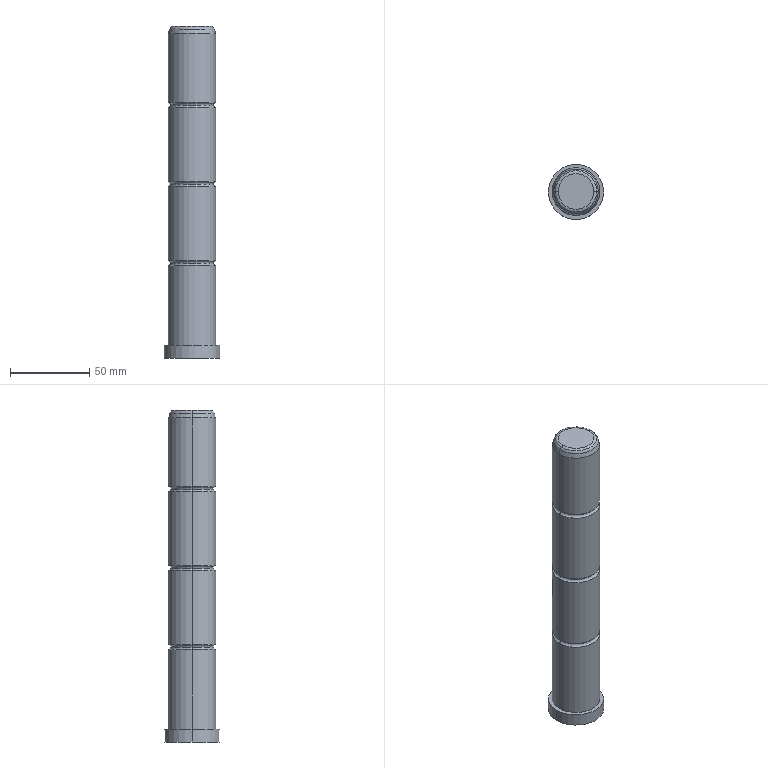Part | Creo | 1 solid | 37 faces | box 35 x 35 x 210 mm | volume 144944 mm3 | torus 16 | cylinder 12 | cone 6 | plane 3 | commonest cylinder face diameters 30 x8 12 x2 35 x2
STEP:
#1=CARTESIAN_POINT('',(-180.,-320.,-197.));
#2=VERTEX_POINT('',#1);
#3=CARTESIAN_POINT('',(-150.,-320.,-197.));
#4=VERTEX_POINT('',#3);
#5=CARTESIAN_POINT('',(-165.,-320.,-197.));
#6=DIRECTION('',(0.,0.,1.));
#7=DIRECTION('',(-1.,0.,0.));
#8=AXIS2_PLACEMENT_3D('',#5,#6,#7);
#9=CIRCLE('',#8,15.);
#10=EDGE_CURVE('',#2,#4,#9,.T.);
#11=ORIENTED_EDGE('',*,*,#10,.T.);
#12=CARTESIAN_POINT('',(-150.,-320.,-244.));
#13=VERTEX_POINT('',#12);
#14=CARTESIAN_POINT('',(-150.,-320.,-244.));
#15=DIRECTION('',(0.,0.,1.));
#16=VECTOR('',#15,47.);
#17=LINE('',#14,#16);
#18=EDGE_CURVE('',#13,#4,#17,.T.);
#19=ORIENTED_EDGE('',*,*,#18,.F.);
#20=CARTESIAN_POINT('',(-180.,-320.,-244.));
#21=VERTEX_POINT('',#20);
#22=CARTESIAN_POINT('',(-165.,-320.,-244.));
#23=DIRECTION('',(0.,0.,-1.));
#24=DIRECTION('',(1.,0.,0.));
#25=AXIS2_PLACEMENT_3D('',#22,#23,#24);
#26=CIRCLE('',#25,15.);
#27=EDGE_CURVE('',#13,#21,#26,.T.);
#28=ORIENTED_EDGE('',*,*,#27,.T.);
#29=CARTESIAN_POINT('',(-180.,-320.,-244.));
#30=DIRECTION('',(0.,0.,1.));
#31=VECTOR('',#30,47.);
#32=LINE('',#29,#31);
#33=EDGE_CURVE('',#21,#2,#32,.T.);
#34=ORIENTED_EDGE('',*,*,#33,.T.);
#35=EDGE_LOOP('',(#11,#19,#28,#34));
#36=FACE_OUTER_BOUND('',#35,.F.);
#37=CARTESIAN_POINT('',(-165.,-320.,-297.5));
#38=DIRECTION('',(0.,0.,1.));
#39=DIRECTION('',(-1.,0.,0.));
#40=AXIS2_PLACEMENT_3D('',#37,#38,#39);
#41=CYLINDRICAL_SURFACE('',#40,15.);
#42=ADVANCED_FACE('',(#36),#41,.T.);
#43=ORIENTED_EDGE('',*,*,#10,.F.);
#44=CARTESIAN_POINT('',(-178.5,-320.,-195.5));
#45=VERTEX_POINT('',#44);
#46=CARTESIAN_POINT('',(-180.,-320.,-195.5));
#47=DIRECTION('',(0.,1.,0.));
#48=DIRECTION('',(1.,0.,0.));
#49=AXIS2_PLACEMENT_3D('',#46,#47,#48);
#50=CIRCLE('',#49,1.5);
#51=EDGE_CURVE('',#45,#2,#50,.T.);
#52=ORIENTED_EDGE('',*,*,#51,.F.);
#53=CARTESIAN_POINT('',(-151.5,-320.,-195.5));
#54=VERTEX_POINT('',#53);
#55=CARTESIAN_POINT('',(-165.,-320.,-195.5));
#56=DIRECTION('',(0.,0.,1.));
#57=DIRECTION('',(-1.,0.,0.));
#58=AXIS2_PLACEMENT_3D('',#55,#56,#57);
#59=CIRCLE('',#58,13.5);
#60=EDGE_CURVE('',#45,#54,#59,.T.);
#61=ORIENTED_EDGE('',*,*,#60,.T.);
#62=CARTESIAN_POINT('',(-150.,-320.,-195.5));
#63=DIRECTION('',(0.,-1.,0.));
#64=DIRECTION('',(-1.,0.,0.));
#65=AXIS2_PLACEMENT_3D('',#62,#63,#64);
#66=CIRCLE('',#65,1.5);
#67=EDGE_CURVE('',#54,#4,#66,.T.);
#68=ORIENTED_EDGE('',*,*,#67,.T.);
#69=EDGE_LOOP('',(#43,#52,#61,#68));
#70=FACE_OUTER_BOUND('',#69,.F.);
#71=CARTESIAN_POINT('',(-165.,-320.,-195.5));
#72=DIRECTION('',(0.,0.,1.));
#73=DIRECTION('',(-1.,0.,0.));
#74=AXIS2_PLACEMENT_3D('',#71,#72,#73);
#75=TOROIDAL_SURFACE('',#74,15.,1.5);
#76=ADVANCED_FACE('',(#70),#75,.F.);
#77=CARTESIAN_POINT('',(-165.,-320.,-197.));
#78=DIRECTION('',(0.,0.,1.));
#79=DIRECTION('',(1.,0.,0.));
#80=AXIS2_PLACEMENT_3D('',#77,#78,#79);
#81=CIRCLE('',#80,15.);
#82=EDGE_CURVE('',#4,#2,#81,.T.);
#83=ORIENTED_EDGE('',*,*,#82,.F.);
#84=ORIENTED_EDGE('',*,*,#67,.F.);
#85=CARTESIAN_POINT('',(-165.,-320.,-195.5));
#86=DIRECTION('',(0.,0.,1.));
#87=DIRECTION('',(1.,0.,0.));
#88=AXIS2_PLACEMENT_3D('',#85,#86,#87);
#89=CIRCLE('',#88,13.5);
#90=EDGE_CURVE('',#54,#45,#89,.T.);
#91=ORIENTED_EDGE('',*,*,#90,.T.);
#92=ORIENTED_EDGE('',*,*,#51,.T.);
#93=EDGE_LOOP('',(#83,#84,#91,#92));
#94=FACE_OUTER_BOUND('',#93,.F.);
#95=CARTESIAN_POINT('',(-165.,-320.,-195.5));
#96=DIRECTION('',(0.,0.,1.));
#97=DIRECTION('',(-1.,0.,0.));
#98=AXIS2_PLACEMENT_3D('',#95,#96,#97);
#99=TOROIDAL_SURFACE('',#98,15.,1.5);
#100=ADVANCED_FACE('',(#94),#99,.F.);
#101=ORIENTED_EDGE('',*,*,#82,.T.);
#102=ORIENTED_EDGE('',*,*,#33,.F.);
#103=CARTESIAN_POINT('',(-165.,-320.,-244.));
#104=DIRECTION('',(0.,0.,-1.));
#105=DIRECTION('',(-1.,0.,0.));
#106=AXIS2_PLACEMENT_3D('',#103,#104,#105);
#107=CIRCLE('',#106,15.);
#108=EDGE_CURVE('',#21,#13,#107,.T.);
#109=ORIENTED_EDGE('',*,*,#108,.T.);
#110=ORIENTED_EDGE('',*,*,#18,.T.);
#111=EDGE_LOOP('',(#101,#102,#109,#110));
#112=FACE_OUTER_BOUND('',#111,.F.);
#113=CARTESIAN_POINT('',(-165.,-320.,-297.5));
#114=DIRECTION('',(0.,0.,1.));
#115=DIRECTION('',(-1.,0.,0.));
#116=AXIS2_PLACEMENT_3D('',#113,#114,#115);
#117=CYLINDRICAL_SURFACE('',#116,15.);
#118=ADVANCED_FACE('',(#112),#117,.T.);
#119=ORIENTED_EDGE('',*,*,#108,.F.);
#120=CARTESIAN_POINT('',(-178.5,-320.,-245.5));
#121=VERTEX_POINT('',#120);
#122=CARTESIAN_POINT('',(-180.,-320.,-245.5));
#123=DIRECTION('',(0.,1.,0.));
#124=DIRECTION('',(0.,0.,1.));
#125=AXIS2_PLACEMENT_3D('',#122,#123,#124);
#126=CIRCLE('',#125,1.5);
#127=EDGE_CURVE('',#21,#121,#126,.T.);
#128=ORIENTED_EDGE('',*,*,#127,.T.);
#129=CARTESIAN_POINT('',(-151.5,-320.,-245.5));
#130=VERTEX_POINT('',#129);
#131=CARTESIAN_POINT('',(-165.,-320.,-245.5));
#132=DIRECTION('',(0.,0.,1.));
#133=DIRECTION('',(1.,0.,0.));
#134=AXIS2_PLACEMENT_3D('',#131,#132,#133);
#135=CIRCLE('',#134,13.5);
#136=EDGE_CURVE('',#130,#121,#135,.T.);
#137=ORIENTED_EDGE('',*,*,#136,.F.);
#138=CARTESIAN_POINT('',(-150.,-320.,-245.5));
#139=DIRECTION('',(0.,-1.,0.));
#140=DIRECTION('',(0.,0.,1.));
#141=AXIS2_PLACEMENT_3D('',#138,#139,#140);
#142=CIRCLE('',#141,1.5);
#143=EDGE_CURVE('',#13,#130,#142,.T.);
#144=ORIENTED_EDGE('',*,*,#143,.F.);
#145=EDGE_LOOP('',(#119,#128,#137,#144));
#146=FACE_OUTER_BOUND('',#145,.F.);
#147=CARTESIAN_POINT('',(-165.,-320.,-245.5));
#148=DIRECTION('',(0.,0.,1.));
#149=DIRECTION('',(-1.,0.,0.));
#150=AXIS2_PLACEMENT_3D('',#147,#148,#149);
#151=TOROIDAL_SURFACE('',#150,15.,1.5);
#152=ADVANCED_FACE('',(#146),#151,.F.);
#153=ORIENTED_EDGE('',*,*,#27,.F.);
#154=ORIENTED_EDGE('',*,*,#143,.T.);
#155=CARTESIAN_POINT('',(-165.,-320.,-245.5));
#156=DIRECTION('',(0.,0.,1.));
#157=DIRECTION('',(-1.,0.,0.));
#158=AXIS2_PLACEMENT_3D('',#155,#156,#157);
#159=CIRCLE('',#158,13.5);
#160=EDGE_CURVE('',#121,#130,#159,.T.);
#161=ORIENTED_EDGE('',*,*,#160,.F.);
#162=ORIENTED_EDGE('',*,*,#127,.F.);
#163=EDGE_LOOP('',(#153,#154,#161,#162));
#164=FACE_OUTER_BOUND('',#163,.F.);
#165=CARTESIAN_POINT('',(-165.,-320.,-245.5));
#166=DIRECTION('',(0.,0.,1.));
#167=DIRECTION('',(-1.,0.,0.));
#168=AXIS2_PLACEMENT_3D('',#165,#166,#167);
#169=TOROIDAL_SURFACE('',#168,15.,1.5);
#170=ADVANCED_FACE('',(#164),#169,.F.);
#171=CARTESIAN_POINT('',(-180.,-320.,-247.));
#172=VERTEX_POINT('',#171);
#173=CARTESIAN_POINT('',(-150.,-320.,-247.));
#174=VERTEX_POINT('',#173);
#175=CARTESIAN_POINT('',(-165.,-320.,-247.));
#176=DIRECTION('',(0.,0.,1.));
#177=DIRECTION('',(-1.,0.,0.));
#178=AXIS2_PLACEMENT_3D('',#175,#176,#177);
#179=CIRCLE('',#178,15.);
#180=EDGE_CURVE('',#172,#174,#179,.T.);
#181=ORIENTED_EDGE('',*,*,#180,.F.);
#182=CARTESIAN_POINT('',(-180.,-320.,-245.5));
#183=DIRECTION('',(0.,1.,0.));
#184=DIRECTION('',(1.,0.,0.));
#185=AXIS2_PLACEMENT_3D('',#182,#183,#184);
#186=CIRCLE('',#185,1.5);
#187=EDGE_CURVE('',#121,#172,#186,.T.);
#188=ORIENTED_EDGE('',*,*,#187,.F.);
#189=ORIENTED_EDGE('',*,*,#160,.T.);
#190=CARTESIAN_POINT('',(-150.,-320.,-245.5));
#191=DIRECTION('',(0.,-1.,0.));
#192=DIRECTION('',(-1.,0.,0.));
#193=AXIS2_PLACEMENT_3D('',#190,#191,#192);
#194=CIRCLE('',#193,1.5);
#195=EDGE_CURVE('',#130,#174,#194,.T.);
#196=ORIENTED_EDGE('',*,*,#195,.T.);
#197=EDGE_LOOP('',(#181,#188,#189,#196));
#198=FACE_OUTER_BOUND('',#197,.F.);
#199=CARTESIAN_POINT('',(-165.,-320.,-245.5));
#200=DIRECTION('',(0.,0.,1.));
#201=DIRECTION('',(-1.,0.,0.));
#202=AXIS2_PLACEMENT_3D('',#199,#200,#201);
#203=TOROIDAL_SURFACE('',#202,15.,1.5);
#204=ADVANCED_FACE('',(#198),#203,.F.);
#205=CARTESIAN_POINT('',(-150.,-320.,-297.5));
#206=VERTEX_POINT('',#205);
#207=CARTESIAN_POINT('',(-180.,-320.,-297.5));
#208=VERTEX_POINT('',#207);
#209=CARTESIAN_POINT('',(-165.,-320.,-297.5));
#210=DIRECTION('',(0.,0.,-1.));
#211=DIRECTION('',(1.,0.,0.));
#212=AXIS2_PLACEMENT_3D('',#209,#210,#211);
#213=CIRCLE('',#212,15.);
#214=EDGE_CURVE('',#206,#208,#213,.T.);
#215=ORIENTED_EDGE('',*,*,#214,.T.);
#216=CARTESIAN_POINT('',(-180.,-320.,-297.5));
#217=DIRECTION('',(0.,0.,1.));
#218=VECTOR('',#217,50.5);
#219=LINE('',#216,#218);
#220=EDGE_CURVE('',#208,#172,#219,.T.);
#221=ORIENTED_EDGE('',*,*,#220,.T.);
#222=ORIENTED_EDGE('',*,*,#180,.T.);
#223=CARTESIAN_POINT('',(-150.,-320.,-297.5));
#224=DIRECTION('',(0.,0.,1.));
#225=VECTOR('',#224,50.5);
#226=LINE('',#223,#225);
#227=EDGE_CURVE('',#206,#174,#226,.T.);
#228=ORIENTED_EDGE('',*,*,#227,.F.);
#229=EDGE_LOOP('',(#215,#221,#222,#228));
#230=FACE_OUTER_BOUND('',#229,.F.);
#231=CARTESIAN_POINT('',(-165.,-320.,-297.5));
#232=DIRECTION('',(0.,0.,1.));
#233=DIRECTION('',(-1.,0.,0.));
#234=AXIS2_PLACEMENT_3D('',#231,#232,#233);
#235=CYLINDRICAL_SURFACE('',#234,15.);
#236=ADVANCED_FACE('',(#230),#235,.T.);
#237=CARTESIAN_POINT('',(-147.5,-320.,-297.5));
#238=VERTEX_POINT('',#237);
#239=CARTESIAN_POINT('',(-182.5,-320.,-297.5));
#240=VERTEX_POINT('',#239);
#241=CARTESIAN_POINT('',(-165.,-320.,-297.5));
#242=DIRECTION('',(0.,0.,1.));
#243=DIRECTION('',(1.,0.,0.));
#244=AXIS2_PLACEMENT_3D('',#241,#242,#243);
#245=CIRCLE('',#244,17.5);
#246=EDGE_CURVE('',#238,#240,#245,.T.);
#247=ORIENTED_EDGE('',*,*,#246,.F.);
#248=CARTESIAN_POINT('',(-165.,-320.,-297.5));
#249=DIRECTION('',(0.,0.,1.));
#250=DIRECTION('',(-1.,0.,0.));
#251=AXIS2_PLACEMENT_3D('',#248,#249,#250);
#252=CIRCLE('',#251,17.5);
#253=EDGE_CURVE('',#240,#238,#252,.T.);
#254=ORIENTED_EDGE('',*,*,#253,.F.);
#255=EDGE_LOOP('',(#247,#254));
#256=FACE_OUTER_BOUND('',#255,.F.);
#257=CARTESIAN_POINT('',(-165.,-320.,-297.5));
#258=DIRECTION('',(0.,0.,-1.));
#259=DIRECTION('',(-1.,0.,0.));
#260=AXIS2_PLACEMENT_3D('',#257,#258,#259);
#261=CIRCLE('',#260,15.);
#262=EDGE_CURVE('',#208,#206,#261,.T.);
#263=ORIENTED_EDGE('',*,*,#262,.F.);
#264=ORIENTED_EDGE('',*,*,#214,.F.);
#265=EDGE_LOOP('',(#263,#264));
#266=FACE_BOUND('',#265,.F.);
#267=CARTESIAN_POINT('',(-165.,-320.,-297.5));
#268=DIRECTION('',(0.,0.,-1.));
#269=DIRECTION('',(1.,0.,0.));
#270=AXIS2_PLACEMENT_3D('',#267,#268,#269);
#271=PLANE('',#270);
#272=ADVANCED_FACE('',(#256,#266),#271,.F.);
#273=ORIENTED_EDGE('',*,*,#262,.T.);
#274=ORIENTED_EDGE('',*,*,#227,.T.);
#275=CARTESIAN_POINT('',(-165.,-320.,-247.));
#276=DIRECTION('',(0.,0.,1.));
#277=DIRECTION('',(1.,0.,0.));
#278=AXIS2_PLACEMENT_3D('',#275,#276,#277);
#279=CIRCLE('',#278,15.);
#280=EDGE_CURVE('',#174,#172,#279,.T.);
#281=ORIENTED_EDGE('',*,*,#280,.T.);
#282=ORIENTED_EDGE('',*,*,#220,.F.);
#283=EDGE_LOOP('',(#273,#274,#281,#282));
#284=FACE_OUTER_BOUND('',#283,.F.);
#285=CARTESIAN_POINT('',(-165.,-320.,-297.5));
#286=DIRECTION('',(0.,0.,1.));
#287=DIRECTION('',(-1.,0.,0.));
#288=AXIS2_PLACEMENT_3D('',#285,#286,#287);
#289=CYLINDRICAL_SURFACE('',#288,15.);
#290=ADVANCED_FACE('',(#284),#289,.T.);
#291=ORIENTED_EDGE('',*,*,#280,.F.);
#292=ORIENTED_EDGE('',*,*,#195,.F.);
#293=ORIENTED_EDGE('',*,*,#136,.T.);
#294=ORIENTED_EDGE('',*,*,#187,.T.);
#295=EDGE_LOOP('',(#291,#292,#293,#294));
#296=FACE_OUTER_BOUND('',#295,.F.);
#297=CARTESIAN_POINT('',(-165.,-320.,-245.5));
#298=DIRECTION('',(0.,0.,1.));
#299=DIRECTION('',(-1.,0.,0.));
#300=AXIS2_PLACEMENT_3D('',#297,#298,#299);
#301=TOROIDAL_SURFACE('',#300,15.,1.5);
#302=ADVANCED_FACE('',(#296),#301,.F.);
#303=ORIENTED_EDGE('',*,*,#246,.T.);
#304=CARTESIAN_POINT('',(-182.5,-320.,-305.5));
#305=VERTEX_POINT('',#304);
#306=CARTESIAN_POINT('',(-182.5,-320.,-297.5));
#307=DIRECTION('',(0.,0.,-1.));
#308=VECTOR('',#307,8.);
#309=LINE('',#306,#308);
#310=EDGE_CURVE('',#240,#305,#309,.T.);
#311=ORIENTED_EDGE('',*,*,#310,.T.);
#312=CARTESIAN_POINT('',(-147.5,-320.,-305.5));
#313=VERTEX_POINT('',#312);
#314=CARTESIAN_POINT('',(-165.,-320.,-305.5));
#315=DIRECTION('',(0.,0.,-1.));
#316=DIRECTION('',(-1.,0.,0.));
#317=AXIS2_PLACEMENT_3D('',#314,#315,#316);
#318=CIRCLE('',#317,17.5);
#319=EDGE_CURVE('',#305,#313,#318,.T.);
#320=ORIENTED_EDGE('',*,*,#319,.T.);
#321=CARTESIAN_POINT('',(-147.5,-320.,-297.5));
#322=DIRECTION('',(0.,0.,-1.));
#323=VECTOR('',#322,8.);
#324=LINE('',#321,#323);
#325=EDGE_CURVE('',#238,#313,#324,.T.);
#326=ORIENTED_EDGE('',*,*,#325,.F.);
#327=EDGE_LOOP('',(#303,#311,#320,#326));
#328=FACE_OUTER_BOUND('',#327,.F.);
#329=CARTESIAN_POINT('',(-165.,-320.,-297.5));
#330=DIRECTION('',(0.,0.,-1.));
#331=DIRECTION('',(1.,0.,0.));
#332=AXIS2_PLACEMENT_3D('',#329,#330,#331);
#333=CYLINDRICAL_SURFACE('',#332,17.5);
#334=ADVANCED_FACE('',(#328),#333,.T.);
#335=ORIENTED_EDGE('',*,*,#253,.T.);
#336=ORIENTED_EDGE('',*,*,#325,.T.);
#337=CARTESIAN_POINT('',(-165.,-320.,-305.5));
#338=DIRECTION('',(0.,0.,-1.));
#339=DIRECTION('',(1.,0.,0.));
#340=AXIS2_PLACEMENT_3D('',#337,#338,#339);
#341=CIRCLE('',#340,17.5);
#342=EDGE_CURVE('',#313,#305,#341,.T.);
#343=ORIENTED_EDGE('',*,*,#342,.T.);
#344=ORIENTED_EDGE('',*,*,#310,.F.);
#345=EDGE_LOOP('',(#335,#336,#343,#344));
#346=FACE_OUTER_BOUND('',#345,.F.);
#347=CARTESIAN_POINT('',(-165.,-320.,-297.5));
#348=DIRECTION('',(0.,0.,-1.));
#349=DIRECTION('',(1.,0.,0.));
#350=AXIS2_PLACEMENT_3D('',#347,#348,#349);
#351=CYLINDRICAL_SURFACE('',#350,17.5);
#352=ADVANCED_FACE('',(#346),#351,.T.);
#353=ORIENTED_EDGE('',*,*,#342,.F.);
#354=ORIENTED_EDGE('',*,*,#319,.F.);
#355=EDGE_LOOP('',(#353,#354));
#356=FACE_OUTER_BOUND('',#355,.F.);
#357=CARTESIAN_POINT('',(-156.5,-320.,-305.5));
#358=VERTEX_POINT('',#357);
#359=CARTESIAN_POINT('',(-173.5,-320.,-305.5));
#360=VERTEX_POINT('',#359);
#361=CARTESIAN_POINT('',(-165.,-320.,-305.5));
#362=DIRECTION('',(0.,0.,1.));
#363=DIRECTION('',(1.,0.,0.));
#364=AXIS2_PLACEMENT_3D('',#361,#362,#363);
#365=CIRCLE('',#364,8.5);
#366=EDGE_CURVE('',#358,#360,#365,.T.);
#367=ORIENTED_EDGE('',*,*,#366,.F.);
#368=CARTESIAN_POINT('',(-165.,-320.,-305.5));
#369=DIRECTION('',(0.,0.,1.));
#370=DIRECTION('',(-1.,0.,0.));
#371=AXIS2_PLACEMENT_3D('',#368,#369,#370);
#372=CIRCLE('',#371,8.5);
#373=EDGE_CURVE('',#360,#358,#372,.T.);
#374=ORIENTED_EDGE('',*,*,#373,.F.);
#375=EDGE_LOOP('',(#367,#374));
#376=FACE_BOUND('',#375,.F.);
#377=CARTESIAN_POINT('',(-165.,-320.,-305.5));
#378=DIRECTION('',(0.,0.,-1.));
#379=DIRECTION('',(1.,0.,0.));
#380=AXIS2_PLACEMENT_3D('',#377,#378,#379);
#381=PLANE('',#380);
#382=ADVANCED_FACE('',(#356,#376),#381,.T.);
#383=CARTESIAN_POINT('',(-159.,-320.,-303.));
#384=VERTEX_POINT('',#383);
#385=CARTESIAN_POINT('',(-171.,-320.,-303.));
#386=VERTEX_POINT('',#385);
#387=CARTESIAN_POINT('',(-165.,-320.,-303.));
#388=DIRECTION('',(0.,0.,1.));
#389=DIRECTION('',(1.,0.,0.));
#390=AXIS2_PLACEMENT_3D('',#387,#388,#389);
#391=CIRCLE('',#390,6.);
#392=EDGE_CURVE('',#384,#386,#391,.T.);
#393=ORIENTED_EDGE('',*,*,#392,.F.);
#394=CARTESIAN_POINT('',(-159.,-320.,-303.));
#395=DIRECTION('',(0.7071,0.,-0.7071));
#396=VECTOR('',#395,3.536);
#397=LINE('',#394,#396);
#398=EDGE_CURVE('',#384,#358,#397,.T.);
#399=ORIENTED_EDGE('',*,*,#398,.T.);
#400=ORIENTED_EDGE('',*,*,#366,.T.);
#401=CARTESIAN_POINT('',(-171.,-320.,-303.));
#402=DIRECTION('',(-0.7071,0.,-0.7071));
#403=VECTOR('',#402,3.536);
#404=LINE('',#401,#403);
#405=EDGE_CURVE('',#386,#360,#404,.T.);
#406=ORIENTED_EDGE('',*,*,#405,.F.);
#407=EDGE_LOOP('',(#393,#399,#400,#406));
#408=FACE_OUTER_BOUND('',#407,.F.);
#409=CARTESIAN_POINT('',(-165.,-320.,-304.25));
#410=DIRECTION('',(0.,0.,-1.));
#411=DIRECTION('',(1.,0.,0.));
#412=AXIS2_PLACEMENT_3D('',#409,#410,#411);
#413=CONICAL_SURFACE('',#412,7.25,45.);
#414=ADVANCED_FACE('',(#408),#413,.F.);
#415=ORIENTED_EDGE('',*,*,#392,.T.);
#416=CARTESIAN_POINT('',(-171.,-320.,-271.087));
#417=VERTEX_POINT('',#416);
#418=CARTESIAN_POINT('',(-171.,-320.,-303.));
#419=DIRECTION('',(0.,0.,1.));
#420=VECTOR('',#419,31.913);
#421=LINE('',#418,#420);
#422=EDGE_CURVE('',#386,#417,#421,.T.);
#423=ORIENTED_EDGE('',*,*,#422,.T.);
#424=CARTESIAN_POINT('',(-159.,-320.,-271.087));
#425=VERTEX_POINT('',#424);
#426=CARTESIAN_POINT('',(-165.,-320.,-271.087));
#427=DIRECTION('',(0.,0.,-1.));
#428=DIRECTION('',(-1.,0.,0.));
#429=AXIS2_PLACEMENT_3D('',#426,#427,#428);
#430=CIRCLE('',#429,6.);
#431=EDGE_CURVE('',#417,#425,#430,.T.);
#432=ORIENTED_EDGE('',*,*,#431,.T.);
#433=CARTESIAN_POINT('',(-159.,-320.,-303.));
#434=DIRECTION('',(0.,0.,1.));
#435=VECTOR('',#434,31.913);
#436=LINE('',#433,#435);
#437=EDGE_CURVE('',#384,#425,#436,.T.);
#438=ORIENTED_EDGE('',*,*,#437,.F.);
#439=EDGE_LOOP('',(#415,#423,#432,#438));
#440=FACE_OUTER_BOUND('',#439,.F.);
#441=CARTESIAN_POINT('',(-165.,-320.,-305.5));
#442=DIRECTION('',(0.,0.,1.));
#443=DIRECTION('',(-1.,0.,0.));
#444=AXIS2_PLACEMENT_3D('',#441,#442,#443);
#445=CYLINDRICAL_SURFACE('',#444,6.);
#446=ADVANCED_FACE('',(#440),#445,.F.);
#447=CARTESIAN_POINT('',(-165.,-320.,-303.));
#448=DIRECTION('',(0.,0.,1.));
#449=DIRECTION('',(-1.,0.,0.));
#450=AXIS2_PLACEMENT_3D('',#447,#448,#449);
#451=CIRCLE('',#450,6.);
#452=EDGE_CURVE('',#386,#384,#451,.T.);
#453=ORIENTED_EDGE('',*,*,#452,.T.);
#454=ORIENTED_EDGE('',*,*,#437,.T.);
#455=CARTESIAN_POINT('',(-165.,-320.,-271.087));
#456=DIRECTION('',(0.,0.,-1.));
#457=DIRECTION('',(1.,0.,0.));
#458=AXIS2_PLACEMENT_3D('',#455,#456,#457);
#459=CIRCLE('',#458,6.);
#460=EDGE_CURVE('',#425,#417,#459,.T.);
#461=ORIENTED_EDGE('',*,*,#460,.T.);
#462=ORIENTED_EDGE('',*,*,#422,.F.);
#463=EDGE_LOOP('',(#453,#454,#461,#462));
#464=FACE_OUTER_BOUND('',#463,.F.);
#465=CARTESIAN_POINT('',(-165.,-320.,-305.5));
#466=DIRECTION('',(0.,0.,1.));
#467=DIRECTION('',(-1.,0.,0.));
#468=AXIS2_PLACEMENT_3D('',#465,#466,#467);
#469=CYLINDRICAL_SURFACE('',#468,6.);
#470=ADVANCED_FACE('',(#464),#469,.F.);
#471=ORIENTED_EDGE('',*,*,#452,.F.);
#472=ORIENTED_EDGE('',*,*,#405,.T.);
#473=ORIENTED_EDGE('',*,*,#373,.T.);
#474=ORIENTED_EDGE('',*,*,#398,.F.);
#475=EDGE_LOOP('',(#471,#472,#473,#474));
#476=FACE_OUTER_BOUND('',#475,.F.);
#477=CARTESIAN_POINT('',(-165.,-320.,-304.25));
#478=DIRECTION('',(0.,0.,-1.));
#479=DIRECTION('',(1.,0.,0.));
#480=AXIS2_PLACEMENT_3D('',#477,#478,#479);
#481=CONICAL_SURFACE('',#480,7.25,45.);
#482=ADVANCED_FACE('',(#476),#481,.F.);
#483=ORIENTED_EDGE('',*,*,#460,.F.);
#484=CARTESIAN_POINT('',(-165.,-320.,-267.482));
#485=VERTEX_POINT('',#484);
#486=CARTESIAN_POINT('',(-165.,-320.,-267.482));
#487=DIRECTION('',(0.8572,0.,-0.515));
#488=VECTOR('',#487,7.);
#489=LINE('',#486,#488);
#490=EDGE_CURVE('',#485,#425,#489,.T.);
#491=ORIENTED_EDGE('',*,*,#490,.F.);
#492=CARTESIAN_POINT('',(-165.,-320.,-267.482));
#493=DIRECTION('',(-0.8572,0.,-0.515));
#494=VECTOR('',#493,7.);
#495=LINE('',#492,#494);
#496=EDGE_CURVE('',#485,#417,#495,.T.);
#497=ORIENTED_EDGE('',*,*,#496,.T.);
#498=EDGE_LOOP('',(#483,#491,#497));
#499=FACE_OUTER_BOUND('',#498,.F.);
#500=CARTESIAN_POINT('',(-165.,-320.,-269.351));
#501=DIRECTION('',(0.,0.,-1.));
#502=DIRECTION('',(1.,0.,0.));
#503=AXIS2_PLACEMENT_3D('',#500,#501,#502);
#504=CONICAL_SURFACE('',#503,3.111,59.);
#505=ADVANCED_FACE('',(#499),#504,.F.);
#506=ORIENTED_EDGE('',*,*,#431,.F.);
#507=ORIENTED_EDGE('',*,*,#496,.F.);
#508=ORIENTED_EDGE('',*,*,#490,.T.);
#509=EDGE_LOOP('',(#506,#507,#508));
#510=FACE_OUTER_BOUND('',#509,.F.);
#511=CARTESIAN_POINT('',(-165.,-320.,-269.351));
#512=DIRECTION('',(0.,0.,-1.));
#513=DIRECTION('',(1.,0.,0.));
#514=AXIS2_PLACEMENT_3D('',#511,#512,#513);
#515=CONICAL_SURFACE('',#514,3.111,59.);
#516=ADVANCED_FACE('',(#510),#515,.F.);
#517=CARTESIAN_POINT('',(-180.,-320.,-194.));
#518=VERTEX_POINT('',#517);
#519=CARTESIAN_POINT('',(-150.,-320.,-194.));
#520=VERTEX_POINT('',#519);
#521=CARTESIAN_POINT('',(-165.,-320.,-194.));
#522=DIRECTION('',(0.,0.,-1.));
#523=DIRECTION('',(-1.,0.,0.));
#524=AXIS2_PLACEMENT_3D('',#521,#522,#523);
#525=CIRCLE('',#524,15.);
#526=EDGE_CURVE('',#518,#520,#525,.T.);
#527=ORIENTED_EDGE('',*,*,#526,.F.);
#528=CARTESIAN_POINT('',(-180.,-320.,-195.5));
#529=DIRECTION('',(0.,1.,0.));
#530=DIRECTION('',(0.,0.,1.));
#531=AXIS2_PLACEMENT_3D('',#528,#529,#530);
#532=CIRCLE('',#531,1.5);
#533=EDGE_CURVE('',#518,#45,#532,.T.);
#534=ORIENTED_EDGE('',*,*,#533,.T.);
#535=ORIENTED_EDGE('',*,*,#90,.F.);
#536=CARTESIAN_POINT('',(-150.,-320.,-195.5));
#537=DIRECTION('',(0.,-1.,0.));
#538=DIRECTION('',(0.,0.,1.));
#539=AXIS2_PLACEMENT_3D('',#536,#537,#538);
#540=CIRCLE('',#539,1.5);
#541=EDGE_CURVE('',#520,#54,#540,.T.);
#542=ORIENTED_EDGE('',*,*,#541,.F.);
#543=EDGE_LOOP('',(#527,#534,#535,#542));
#544=FACE_OUTER_BOUND('',#543,.F.);
#545=CARTESIAN_POINT('',(-165.,-320.,-195.5));
#546=DIRECTION('',(0.,0.,1.));
#547=DIRECTION('',(-1.,0.,0.));
#548=AXIS2_PLACEMENT_3D('',#545,#546,#547);
#549=TOROIDAL_SURFACE('',#548,15.,1.5);
#550=ADVANCED_FACE('',(#544),#549,.F.);
#551=CARTESIAN_POINT('',(-150.,-320.,-147.));
#552=VERTEX_POINT('',#551);
#553=CARTESIAN_POINT('',(-180.,-320.,-147.));
#554=VERTEX_POINT('',#553);
#555=CARTESIAN_POINT('',(-165.,-320.,-147.));
#556=DIRECTION('',(0.,0.,1.));
#557=DIRECTION('',(1.,0.,0.));
#558=AXIS2_PLACEMENT_3D('',#555,#556,#557);
#559=CIRCLE('',#558,15.);
#560=EDGE_CURVE('',#552,#554,#559,.T.);
#561=ORIENTED_EDGE('',*,*,#560,.T.);
#562=CARTESIAN_POINT('',(-180.,-320.,-194.));
#563=DIRECTION('',(0.,0.,1.));
#564=VECTOR('',#563,47.);
#565=LINE('',#562,#564);
#566=EDGE_CURVE('',#518,#554,#565,.T.);
#567=ORIENTED_EDGE('',*,*,#566,.F.);
#568=ORIENTED_EDGE('',*,*,#526,.T.);
#569=CARTESIAN_POINT('',(-150.,-320.,-194.));
#570=DIRECTION('',(0.,0.,1.));
#571=VECTOR('',#570,47.);
#572=LINE('',#569,#571);
#573=EDGE_CURVE('',#520,#552,#572,.T.);
#574=ORIENTED_EDGE('',*,*,#573,.T.);
#575=EDGE_LOOP('',(#561,#567,#568,#574));
#576=FACE_OUTER_BOUND('',#575,.F.);
#577=CARTESIAN_POINT('',(-165.,-320.,-297.5));
#578=DIRECTION('',(0.,0.,1.));
#579=DIRECTION('',(-1.,0.,0.));
#580=AXIS2_PLACEMENT_3D('',#577,#578,#579);
#581=CYLINDRICAL_SURFACE('',#580,15.);
#582=ADVANCED_FACE('',(#576),#581,.T.);
#583=ORIENTED_EDGE('',*,*,#560,.F.);
#584=CARTESIAN_POINT('',(-151.5,-320.,-145.5));
#585=VERTEX_POINT('',#584);
#586=CARTESIAN_POINT('',(-150.,-320.,-145.5));
#587=DIRECTION('',(0.,-1.,0.));
#588=DIRECTION('',(-1.,0.,0.));
#589=AXIS2_PLACEMENT_3D('',#586,#587,#588);
#590=CIRCLE('',#589,1.5);
#591=EDGE_CURVE('',#585,#552,#590,.T.);
#592=ORIENTED_EDGE('',*,*,#591,.F.);
#593=CARTESIAN_POINT('',(-178.5,-320.,-145.5));
#594=VERTEX_POINT('',#593);
#595=CARTESIAN_POINT('',(-165.,-320.,-145.5));
#596=DIRECTION('',(0.,0.,1.));
#597=DIRECTION('',(1.,0.,0.));
#598=AXIS2_PLACEMENT_3D('',#595,#596,#597);
#599=CIRCLE('',#598,13.5);
#600=EDGE_CURVE('',#585,#594,#599,.T.);
#601=ORIENTED_EDGE('',*,*,#600,.T.);
#602=CARTESIAN_POINT('',(-180.,-320.,-145.5));
#603=DIRECTION('',(0.,1.,0.));
#604=DIRECTION('',(1.,0.,0.));
#605=AXIS2_PLACEMENT_3D('',#602,#603,#604);
#606=CIRCLE('',#605,1.5);
#607=EDGE_CURVE('',#594,#554,#606,.T.);
#608=ORIENTED_EDGE('',*,*,#607,.T.);
#609=EDGE_LOOP('',(#583,#592,#601,#608));
#610=FACE_OUTER_BOUND('',#609,.F.);
#611=CARTESIAN_POINT('',(-165.,-320.,-145.5));
#612=DIRECTION('',(0.,0.,1.));
#613=DIRECTION('',(-1.,0.,0.));
#614=AXIS2_PLACEMENT_3D('',#611,#612,#613);
#615=TOROIDAL_SURFACE('',#614,15.,1.5);
#616=ADVANCED_FACE('',(#610),#615,.F.);
#617=CARTESIAN_POINT('',(-165.,-320.,-147.));
#618=DIRECTION('',(0.,0.,1.));
#619=DIRECTION('',(-1.,0.,0.));
#620=AXIS2_PLACEMENT_3D('',#617,#618,#619);
#621=CIRCLE('',#620,15.);
#622=EDGE_CURVE('',#554,#552,#621,.T.);
#623=ORIENTED_EDGE('',*,*,#622,.F.);
#624=ORIENTED_EDGE('',*,*,#607,.F.);
#625=CARTESIAN_POINT('',(-165.,-320.,-145.5));
#626=DIRECTION('',(0.,0.,1.));
#627=DIRECTION('',(-1.,0.,0.));
#628=AXIS2_PLACEMENT_3D('',#625,#626,#627);
#629=CIRCLE('',#628,13.5);
#630=EDGE_CURVE('',#594,#585,#629,.T.);
#631=ORIENTED_EDGE('',*,*,#630,.T.);
#632=ORIENTED_EDGE('',*,*,#591,.T.);
#633=EDGE_LOOP('',(#623,#624,#631,#632));
#634=FACE_OUTER_BOUND('',#633,.F.);
#635=CARTESIAN_POINT('',(-165.,-320.,-145.5));
#636=DIRECTION('',(0.,0.,1.));
#637=DIRECTION('',(-1.,0.,0.));
#638=AXIS2_PLACEMENT_3D('',#635,#636,#637);
#639=TOROIDAL_SURFACE('',#638,15.,1.5);
#640=ADVANCED_FACE('',(#634),#639,.F.);
#641=ORIENTED_EDGE('',*,*,#622,.T.);
#642=ORIENTED_EDGE('',*,*,#573,.F.);
#643=CARTESIAN_POINT('',(-165.,-320.,-194.));
#644=DIRECTION('',(0.,0.,-1.));
#645=DIRECTION('',(1.,0.,0.));
#646=AXIS2_PLACEMENT_3D('',#643,#644,#645);
#647=CIRCLE('',#646,15.);
#648=EDGE_CURVE('',#520,#518,#647,.T.);
#649=ORIENTED_EDGE('',*,*,#648,.T.);
#650=ORIENTED_EDGE('',*,*,#566,.T.);
#651=EDGE_LOOP('',(#641,#642,#649,#650));
#652=FACE_OUTER_BOUND('',#651,.F.);
#653=CARTESIAN_POINT('',(-165.,-320.,-297.5));
#654=DIRECTION('',(0.,0.,1.));
#655=DIRECTION('',(-1.,0.,0.));
#656=AXIS2_PLACEMENT_3D('',#653,#654,#655);
#657=CYLINDRICAL_SURFACE('',#656,15.);
#658=ADVANCED_FACE('',(#652),#657,.T.);
#659=ORIENTED_EDGE('',*,*,#648,.F.);
#660=ORIENTED_EDGE('',*,*,#541,.T.);
#661=ORIENTED_EDGE('',*,*,#60,.F.);
#662=ORIENTED_EDGE('',*,*,#533,.F.);
#663=EDGE_LOOP('',(#659,#660,#661,#662));
#664=FACE_OUTER_BOUND('',#663,.F.);
#665=CARTESIAN_POINT('',(-165.,-320.,-195.5));
#666=DIRECTION('',(0.,0.,1.));
#667=DIRECTION('',(-1.,0.,0.));
#668=AXIS2_PLACEMENT_3D('',#665,#666,#667);
#669=TOROIDAL_SURFACE('',#668,15.,1.5);
#670=ADVANCED_FACE('',(#664),#669,.F.);
#671=CARTESIAN_POINT('',(-150.,-320.,-144.));
#672=VERTEX_POINT('',#671);
#673=CARTESIAN_POINT('',(-180.,-320.,-144.));
#674=VERTEX_POINT('',#673);
#675=CARTESIAN_POINT('',(-165.,-320.,-144.));
#676=DIRECTION('',(0.,0.,-1.));
#677=DIRECTION('',(1.,0.,0.));
#678=AXIS2_PLACEMENT_3D('',#675,#676,#677);
#679=CIRCLE('',#678,15.);
#680=EDGE_CURVE('',#672,#674,#679,.T.);
#681=ORIENTED_EDGE('',*,*,#680,.F.);
#682=CARTESIAN_POINT('',(-150.,-320.,-145.5));
#683=DIRECTION('',(0.,-1.,0.));
#684=DIRECTION('',(0.,0.,1.));
#685=AXIS2_PLACEMENT_3D('',#682,#683,#684);
#686=CIRCLE('',#685,1.5);
#687=EDGE_CURVE('',#672,#585,#686,.T.);
#688=ORIENTED_EDGE('',*,*,#687,.T.);
#689=ORIENTED_EDGE('',*,*,#630,.F.);
#690=CARTESIAN_POINT('',(-180.,-320.,-145.5));
#691=DIRECTION('',(0.,1.,0.));
#692=DIRECTION('',(0.,0.,1.));
#693=AXIS2_PLACEMENT_3D('',#690,#691,#692);
#694=CIRCLE('',#693,1.5);
#695=EDGE_CURVE('',#674,#594,#694,.T.);
#696=ORIENTED_EDGE('',*,*,#695,.F.);
#697=EDGE_LOOP('',(#681,#688,#689,#696));
#698=FACE_OUTER_BOUND('',#697,.F.);
#699=CARTESIAN_POINT('',(-165.,-320.,-145.5));
#700=DIRECTION('',(0.,0.,1.));
#701=DIRECTION('',(-1.,0.,0.));
#702=AXIS2_PLACEMENT_3D('',#699,#700,#701);
#703=TOROIDAL_SURFACE('',#702,15.,1.5);
#704=ADVANCED_FACE('',(#698),#703,.F.);
#705=ORIENTED_EDGE('',*,*,#680,.T.);
#706=CARTESIAN_POINT('',(-180.,-320.,-100.5));
#707=VERTEX_POINT('',#706);
#708=CARTESIAN_POINT('',(-180.,-320.,-144.));
#709=DIRECTION('',(0.,0.,1.));
#710=VECTOR('',#709,43.5);
#711=LINE('',#708,#710);
#712=EDGE_CURVE('',#674,#707,#711,.T.);
#713=ORIENTED_EDGE('',*,*,#712,.T.);
#714=CARTESIAN_POINT('',(-150.,-320.,-100.5));
#715=VERTEX_POINT('',#714);
#716=CARTESIAN_POINT('',(-165.,-320.,-100.5));
#717=DIRECTION('',(0.,0.,1.));
#718=DIRECTION('',(-1.,0.,0.));
#719=AXIS2_PLACEMENT_3D('',#716,#717,#718);
#720=CIRCLE('',#719,15.);
#721=EDGE_CURVE('',#707,#715,#720,.T.);
#722=ORIENTED_EDGE('',*,*,#721,.T.);
#723=CARTESIAN_POINT('',(-150.,-320.,-144.));
#724=DIRECTION('',(0.,0.,1.));
#725=VECTOR('',#724,43.5);
#726=LINE('',#723,#725);
#727=EDGE_CURVE('',#672,#715,#726,.T.);
#728=ORIENTED_EDGE('',*,*,#727,.F.);
#729=EDGE_LOOP('',(#705,#713,#722,#728));
#730=FACE_OUTER_BOUND('',#729,.F.);
#731=CARTESIAN_POINT('',(-165.,-320.,-297.5));
#732=DIRECTION('',(0.,0.,1.));
#733=DIRECTION('',(-1.,0.,0.));
#734=AXIS2_PLACEMENT_3D('',#731,#732,#733);
#735=CYLINDRICAL_SURFACE('',#734,15.);
#736=ADVANCED_FACE('',(#730),#735,.T.);
#737=CARTESIAN_POINT('',(-165.,-320.,-144.));
#738=DIRECTION('',(0.,0.,-1.));
#739=DIRECTION('',(-1.,0.,0.));
#740=AXIS2_PLACEMENT_3D('',#737,#738,#739);
#741=CIRCLE('',#740,15.);
#742=EDGE_CURVE('',#674,#672,#741,.T.);
#743=ORIENTED_EDGE('',*,*,#742,.T.);
#744=ORIENTED_EDGE('',*,*,#727,.T.);
#745=CARTESIAN_POINT('',(-165.,-320.,-100.5));
#746=DIRECTION('',(0.,0.,1.));
#747=DIRECTION('',(1.,0.,0.));
#748=AXIS2_PLACEMENT_3D('',#745,#746,#747);
#749=CIRCLE('',#748,15.);
#750=EDGE_CURVE('',#715,#707,#749,.T.);
#751=ORIENTED_EDGE('',*,*,#750,.T.);
#752=ORIENTED_EDGE('',*,*,#712,.F.);
#753=EDGE_LOOP('',(#743,#744,#751,#752));
#754=FACE_OUTER_BOUND('',#753,.F.);
#755=CARTESIAN_POINT('',(-165.,-320.,-297.5));
#756=DIRECTION('',(0.,0.,1.));
#757=DIRECTION('',(-1.,0.,0.));
#758=AXIS2_PLACEMENT_3D('',#755,#756,#757);
#759=CYLINDRICAL_SURFACE('',#758,15.);
#760=ADVANCED_FACE('',(#754),#759,.T.);
#761=ORIENTED_EDGE('',*,*,#742,.F.);
#762=ORIENTED_EDGE('',*,*,#695,.T.);
#763=ORIENTED_EDGE('',*,*,#600,.F.);
#764=ORIENTED_EDGE('',*,*,#687,.F.);
#765=EDGE_LOOP('',(#761,#762,#763,#764));
#766=FACE_OUTER_BOUND('',#765,.F.);
#767=CARTESIAN_POINT('',(-165.,-320.,-145.5));
#768=DIRECTION('',(0.,0.,1.));
#769=DIRECTION('',(-1.,0.,0.));
#770=AXIS2_PLACEMENT_3D('',#767,#768,#769);
#771=TOROIDAL_SURFACE('',#770,15.,1.5);
#772=ADVANCED_FACE('',(#766),#771,.F.);
#773=CARTESIAN_POINT('',(-150.859,-320.,-97.638));
#774=VERTEX_POINT('',#773);
#775=CARTESIAN_POINT('',(-179.141,-320.,-97.638));
#776=VERTEX_POINT('',#775);
#777=CARTESIAN_POINT('',(-165.,-320.,-97.638));
#778=DIRECTION('',(0.,0.,1.));
#779=DIRECTION('',(1.,0.,0.));
#780=AXIS2_PLACEMENT_3D('',#777,#778,#779);
#781=CIRCLE('',#780,14.141);
#782=EDGE_CURVE('',#774,#776,#781,.T.);
#783=ORIENTED_EDGE('',*,*,#782,.T.);
#784=CARTESIAN_POINT('',(-179.141,-320.,-97.638));
#785=DIRECTION('',(-0.2873,0.,-0.9578));
#786=VECTOR('',#785,2.988);
#787=LINE('',#784,#786);
#788=EDGE_CURVE('',#776,#707,#787,.T.);
#789=ORIENTED_EDGE('',*,*,#788,.T.);
#790=ORIENTED_EDGE('',*,*,#750,.F.);
#791=CARTESIAN_POINT('',(-150.859,-320.,-97.638));
#792=DIRECTION('',(0.2873,0.,-0.9578));
#793=VECTOR('',#792,2.988);
#794=LINE('',#791,#793);
#795=EDGE_CURVE('',#774,#715,#794,.T.);
#796=ORIENTED_EDGE('',*,*,#795,.F.);
#797=EDGE_LOOP('',(#783,#789,#790,#796));
#798=FACE_OUTER_BOUND('',#797,.F.);
#799=CARTESIAN_POINT('',(-165.,-320.,-99.069));
#800=DIRECTION('',(0.,0.,-1.));
#801=DIRECTION('',(1.,0.,0.));
#802=AXIS2_PLACEMENT_3D('',#799,#800,#801);
#803=CONICAL_SURFACE('',#802,14.571,16.699);
#804=ADVANCED_FACE('',(#798),#803,.T.);
#805=ORIENTED_EDGE('',*,*,#782,.F.);
#806=CARTESIAN_POINT('',(-151.941,-320.,-96.093));
#807=VERTEX_POINT('',#806);
#808=CARTESIAN_POINT('',(-153.732,-320.,-98.5));
#809=DIRECTION('',(0.,-1.,0.));
#810=DIRECTION('',(0.9578,0.,0.2873));
#811=AXIS2_PLACEMENT_3D('',#808,#809,#810);
#812=CIRCLE('',#811,3.);
#813=EDGE_CURVE('',#774,#807,#812,.T.);
#814=ORIENTED_EDGE('',*,*,#813,.T.);
#815=CARTESIAN_POINT('',(-178.059,-320.,-96.093));
#816=VERTEX_POINT('',#815);
#817=CARTESIAN_POINT('',(-165.,-320.,-96.093));
#818=DIRECTION('',(0.,0.,1.));
#819=DIRECTION('',(1.,0.,0.));
#820=AXIS2_PLACEMENT_3D('',#817,#818,#819);
#821=CIRCLE('',#820,13.059);
#822=EDGE_CURVE('',#807,#816,#821,.T.);
#823=ORIENTED_EDGE('',*,*,#822,.T.);
#824=CARTESIAN_POINT('',(-176.268,-320.,-98.5));
#825=DIRECTION('',(0.,1.,0.));
#826=DIRECTION('',(-0.9578,0.,0.2873));
#827=AXIS2_PLACEMENT_3D('',#824,#825,#826);
#828=CIRCLE('',#827,3.);
#829=EDGE_CURVE('',#776,#816,#828,.T.);
#830=ORIENTED_EDGE('',*,*,#829,.F.);
#831=EDGE_LOOP('',(#805,#814,#823,#830));
#832=FACE_OUTER_BOUND('',#831,.F.);
#833=CARTESIAN_POINT('',(-165.,-320.,-98.5));
#834=DIRECTION('',(0.,0.,1.));
#835=DIRECTION('',(-1.,0.,0.));
#836=AXIS2_PLACEMENT_3D('',#833,#834,#835);
#837=TOROIDAL_SURFACE('',#836,11.268,3.);
#838=ADVANCED_FACE('',(#832),#837,.T.);
#839=CARTESIAN_POINT('',(-165.,-320.,-97.638));
#840=DIRECTION('',(0.,0.,1.));
#841=DIRECTION('',(-1.,0.,0.));
#842=AXIS2_PLACEMENT_3D('',#839,#840,#841);
#843=CIRCLE('',#842,14.141);
#844=EDGE_CURVE('',#776,#774,#843,.T.);
#845=ORIENTED_EDGE('',*,*,#844,.F.);
#846=ORIENTED_EDGE('',*,*,#829,.T.);
#847=CARTESIAN_POINT('',(-165.,-320.,-96.093));
#848=DIRECTION('',(0.,0.,1.));
#849=DIRECTION('',(-1.,0.,0.));
#850=AXIS2_PLACEMENT_3D('',#847,#848,#849);
#851=CIRCLE('',#850,13.059);
#852=EDGE_CURVE('',#816,#807,#851,.T.);
#853=ORIENTED_EDGE('',*,*,#852,.T.);
#854=ORIENTED_EDGE('',*,*,#813,.F.);
#855=EDGE_LOOP('',(#845,#846,#853,#854));
#856=FACE_OUTER_BOUND('',#855,.F.);
#857=CARTESIAN_POINT('',(-165.,-320.,-98.5));
#858=DIRECTION('',(0.,0.,1.));
#859=DIRECTION('',(-1.,0.,0.));
#860=AXIS2_PLACEMENT_3D('',#857,#858,#859);
#861=TOROIDAL_SURFACE('',#860,11.268,3.);
#862=ADVANCED_FACE('',(#856),#861,.T.);
#863=ORIENTED_EDGE('',*,*,#844,.T.);
#864=ORIENTED_EDGE('',*,*,#795,.T.);
#865=ORIENTED_EDGE('',*,*,#721,.F.);
#866=ORIENTED_EDGE('',*,*,#788,.F.);
#867=EDGE_LOOP('',(#863,#864,#865,#866));
#868=FACE_OUTER_BOUND('',#867,.F.);
#869=CARTESIAN_POINT('',(-165.,-320.,-99.069));
#870=DIRECTION('',(0.,0.,-1.));
#871=DIRECTION('',(1.,0.,0.));
#872=AXIS2_PLACEMENT_3D('',#869,#870,#871);
#873=CONICAL_SURFACE('',#872,14.571,16.699);
#874=ADVANCED_FACE('',(#868),#873,.T.);
#875=CARTESIAN_POINT('',(-176.268,-320.,-95.5));
#876=VERTEX_POINT('',#875);
#877=CARTESIAN_POINT('',(-153.732,-320.,-95.5));
#878=VERTEX_POINT('',#877);
#879=CARTESIAN_POINT('',(-165.,-320.,-95.5));
#880=DIRECTION('',(0.,0.,1.));
#881=DIRECTION('',(-1.,0.,0.));
#882=AXIS2_PLACEMENT_3D('',#879,#880,#881);
#883=CIRCLE('',#882,11.268);
#884=EDGE_CURVE('',#876,#878,#883,.T.);
#885=ORIENTED_EDGE('',*,*,#884,.T.);
#886=CARTESIAN_POINT('',(-153.732,-320.,-98.5));
#887=DIRECTION('',(0.,-1.,0.));
#888=DIRECTION('',(0.5969,0.,0.8023));
#889=AXIS2_PLACEMENT_3D('',#886,#887,#888);
#890=CIRCLE('',#889,3.);
#891=EDGE_CURVE('',#807,#878,#890,.T.);
#892=ORIENTED_EDGE('',*,*,#891,.F.);
#893=ORIENTED_EDGE('',*,*,#852,.F.);
#894=CARTESIAN_POINT('',(-176.268,-320.,-98.5));
#895=DIRECTION('',(0.,1.,0.));
#896=DIRECTION('',(-0.5969,0.,0.8023));
#897=AXIS2_PLACEMENT_3D('',#894,#895,#896);
#898=CIRCLE('',#897,3.);
#899=EDGE_CURVE('',#816,#876,#898,.T.);
#900=ORIENTED_EDGE('',*,*,#899,.T.);
#901=EDGE_LOOP('',(#885,#892,#893,#900));
#902=FACE_OUTER_BOUND('',#901,.F.);
#903=CARTESIAN_POINT('',(-165.,-320.,-98.5));
#904=DIRECTION('',(0.,0.,1.));
#905=DIRECTION('',(-1.,0.,0.));
#906=AXIS2_PLACEMENT_3D('',#903,#904,#905);
#907=TOROIDAL_SURFACE('',#906,11.268,3.);
#908=ADVANCED_FACE('',(#902),#907,.T.);
#909=ORIENTED_EDGE('',*,*,#884,.F.);
#910=CARTESIAN_POINT('',(-165.,-320.,-95.5));
#911=DIRECTION('',(0.,0.,1.));
#912=DIRECTION('',(1.,0.,0.));
#913=AXIS2_PLACEMENT_3D('',#910,#911,#912);
#914=CIRCLE('',#913,11.268);
#915=EDGE_CURVE('',#878,#876,#914,.T.);
#916=ORIENTED_EDGE('',*,*,#915,.F.);
#917=EDGE_LOOP('',(#909,#916));
#918=FACE_OUTER_BOUND('',#917,.F.);
#919=CARTESIAN_POINT('',(-165.,-320.,-95.5));
#920=DIRECTION('',(0.,0.,1.));
#921=DIRECTION('',(-1.,0.,0.));
#922=AXIS2_PLACEMENT_3D('',#919,#920,#921);
#923=PLANE('',#922);
#924=ADVANCED_FACE('',(#918),#923,.T.);
#925=ORIENTED_EDGE('',*,*,#915,.T.);
#926=ORIENTED_EDGE('',*,*,#899,.F.);
#927=ORIENTED_EDGE('',*,*,#822,.F.);
#928=ORIENTED_EDGE('',*,*,#891,.T.);
#929=EDGE_LOOP('',(#925,#926,#927,#928));
#930=FACE_OUTER_BOUND('',#929,.F.);
#931=CARTESIAN_POINT('',(-165.,-320.,-98.5));
#932=DIRECTION('',(0.,0.,1.));
#933=DIRECTION('',(-1.,0.,0.));
#934=AXIS2_PLACEMENT_3D('',#931,#932,#933);
#935=TOROIDAL_SURFACE('',#934,11.268,3.);
#936=ADVANCED_FACE('',(#930),#935,.T.);
#937=CLOSED_SHELL('',(#42,#76,#100,#118,#152,#170,#204,#236,#272,#290,#302,#334,#352,#382,#414,#446,#470,#482,#505,#516,#550,#582,#616,#640,#658,#670,#704,#736,#760,#772,#804,#838,#862,#874,#908,#924,#936));
#938=MANIFOLD_SOLID_BREP('',#937);
#939=(LENGTH_UNIT()NAMED_UNIT(*)SI_UNIT(.MILLI.,.METRE.));
#940=UNCERTAINTY_MEASURE_WITH_UNIT(LENGTH_MEASURE(0.02157),#939,'','');
#941=(NAMED_UNIT(*)PLANE_ANGLE_UNIT()SI_UNIT($,.RADIAN.));
#942=PLANE_ANGLE_MEASURE_WITH_UNIT(PLANE_ANGLE_MEASURE(0.01745),#941);
#943=(CONVERSION_BASED_UNIT('DEGREE',#942)NAMED_UNIT(*)PLANE_ANGLE_UNIT());
#944=(NAMED_UNIT(*)SI_UNIT($,.STERADIAN.)SOLID_ANGLE_UNIT());
#945=(GEOMETRIC_REPRESENTATION_CONTEXT(3)GLOBAL_UNCERTAINTY_ASSIGNED_CONTEXT((#940))GLOBAL_UNIT_ASSIGNED_CONTEXT((#939,#943,#944))REPRESENTATION_CONTEXT('',''));
#946=ADVANCED_BREP_SHAPE_REPRESENTATION('',(#938),#945);